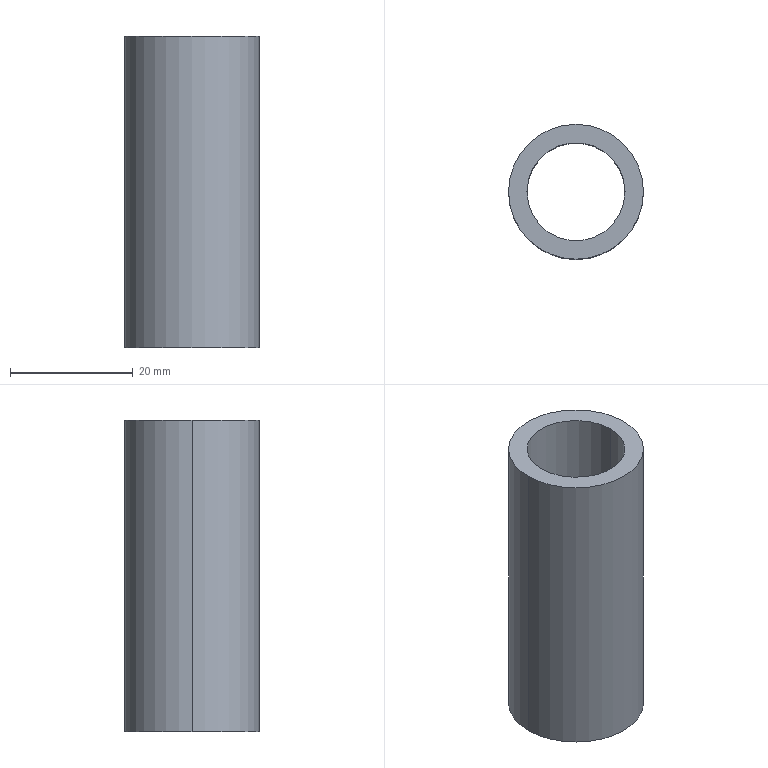Part | SolidWorks | features Extrusion 1 | 1 solid | 6 faces | box 22 x 22 x 50.8 mm | volume 9097 mm3 | cylinder 4 | plane 2 | commonest cylinder face diameters 16 x2 22 x2
STEP:
#1=CARTESIAN_POINT('',(-8.,0.,50.8));
#2=VERTEX_POINT('',#1);
#3=CARTESIAN_POINT('',(8.,0.,50.8));
#4=VERTEX_POINT('',#3);
#5=CARTESIAN_POINT('',(0.,0.,50.8));
#6=DIRECTION('',(0.,0.,1.));
#7=DIRECTION('',(1.,0.,0.));
#8=AXIS2_PLACEMENT_3D('',#5,#6,#7);
#9=CIRCLE('',#8,8.);
#10=EDGE_CURVE('',#2,#4,#9,.T.);
#11=ORIENTED_EDGE('',*,*,#10,.T.);
#12=CARTESIAN_POINT('',(8.,0.,0.));
#13=VERTEX_POINT('',#12);
#14=CARTESIAN_POINT('',(8.,0.,50.8));
#15=DIRECTION('',(0.,0.,-1.));
#16=VECTOR('',#15,1000.);
#17=LINE('',#14,#16);
#18=EDGE_CURVE('',#4,#13,#17,.T.);
#19=ORIENTED_EDGE('',*,*,#18,.T.);
#20=CARTESIAN_POINT('',(-8.,0.,0.));
#21=VERTEX_POINT('',#20);
#22=CARTESIAN_POINT('',(0.,0.,0.));
#23=DIRECTION('',(0.,0.,1.));
#24=DIRECTION('',(1.,0.,0.));
#25=AXIS2_PLACEMENT_3D('',#22,#23,#24);
#26=CIRCLE('',#25,8.);
#27=EDGE_CURVE('',#21,#13,#26,.T.);
#28=ORIENTED_EDGE('',*,*,#27,.F.);
#29=CARTESIAN_POINT('',(-8.,0.,50.8));
#30=DIRECTION('',(0.,0.,-1.));
#31=VECTOR('',#30,1000.);
#32=LINE('',#29,#31);
#33=EDGE_CURVE('',#2,#21,#32,.T.);
#34=ORIENTED_EDGE('',*,*,#33,.F.);
#35=EDGE_LOOP('',(#11,#19,#28,#34));
#36=FACE_OUTER_BOUND('',#35,.T.);
#37=CARTESIAN_POINT('',(0.,0.,50.8));
#38=DIRECTION('',(0.,0.,-1.));
#39=DIRECTION('',(-1.,0.,0.));
#40=AXIS2_PLACEMENT_3D('',#37,#38,#39);
#41=CYLINDRICAL_SURFACE('',#40,8.);
#42=ADVANCED_FACE('',(#36),#41,.F.);
#43=CARTESIAN_POINT('',(11.,0.,50.8));
#44=VERTEX_POINT('',#43);
#45=CARTESIAN_POINT('',(-11.,0.,50.8));
#46=VERTEX_POINT('',#45);
#47=CARTESIAN_POINT('',(0.,0.,50.8));
#48=DIRECTION('',(0.,0.,1.));
#49=DIRECTION('',(1.,0.,0.));
#50=AXIS2_PLACEMENT_3D('',#47,#48,#49);
#51=CIRCLE('',#50,11.);
#52=EDGE_CURVE('',#44,#46,#51,.T.);
#53=ORIENTED_EDGE('',*,*,#52,.F.);
#54=CARTESIAN_POINT('',(11.,0.,0.));
#55=VERTEX_POINT('',#54);
#56=CARTESIAN_POINT('',(11.,0.,50.8));
#57=DIRECTION('',(0.,0.,-1.));
#58=VECTOR('',#57,1000.);
#59=LINE('',#56,#58);
#60=EDGE_CURVE('',#44,#55,#59,.T.);
#61=ORIENTED_EDGE('',*,*,#60,.T.);
#62=CARTESIAN_POINT('',(-11.,0.,0.));
#63=VERTEX_POINT('',#62);
#64=CARTESIAN_POINT('',(0.,0.,0.));
#65=DIRECTION('',(0.,0.,1.));
#66=DIRECTION('',(1.,0.,0.));
#67=AXIS2_PLACEMENT_3D('',#64,#65,#66);
#68=CIRCLE('',#67,11.);
#69=EDGE_CURVE('',#55,#63,#68,.T.);
#70=ORIENTED_EDGE('',*,*,#69,.T.);
#71=CARTESIAN_POINT('',(-11.,0.,50.8));
#72=DIRECTION('',(0.,0.,-1.));
#73=VECTOR('',#72,1000.);
#74=LINE('',#71,#73);
#75=EDGE_CURVE('',#46,#63,#74,.T.);
#76=ORIENTED_EDGE('',*,*,#75,.F.);
#77=EDGE_LOOP('',(#53,#61,#70,#76));
#78=FACE_OUTER_BOUND('',#77,.T.);
#79=CARTESIAN_POINT('',(0.,0.,50.8));
#80=DIRECTION('',(0.,0.,-1.));
#81=DIRECTION('',(-1.,0.,0.));
#82=AXIS2_PLACEMENT_3D('',#79,#80,#81);
#83=CYLINDRICAL_SURFACE('',#82,11.);
#84=ADVANCED_FACE('',(#78),#83,.T.);
#85=CARTESIAN_POINT('',(0.,0.,50.8));
#86=DIRECTION('',(0.,0.,1.));
#87=DIRECTION('',(1.,0.,0.));
#88=AXIS2_PLACEMENT_3D('',#85,#86,#87);
#89=CIRCLE('',#88,11.);
#90=EDGE_CURVE('',#46,#44,#89,.T.);
#91=ORIENTED_EDGE('',*,*,#90,.T.);
#92=ORIENTED_EDGE('',*,*,#52,.T.);
#93=EDGE_LOOP('',(#91,#92));
#94=FACE_OUTER_BOUND('',#93,.T.);
#95=ORIENTED_EDGE('',*,*,#10,.F.);
#96=CARTESIAN_POINT('',(0.,0.,50.8));
#97=DIRECTION('',(0.,0.,1.));
#98=DIRECTION('',(1.,0.,0.));
#99=AXIS2_PLACEMENT_3D('',#96,#97,#98);
#100=CIRCLE('',#99,8.);
#101=EDGE_CURVE('',#4,#2,#100,.T.);
#102=ORIENTED_EDGE('',*,*,#101,.F.);
#103=EDGE_LOOP('',(#95,#102));
#104=FACE_BOUND('',#103,.T.);
#105=CARTESIAN_POINT('',(0.,0.,50.8));
#106=DIRECTION('',(0.,0.,1.));
#107=DIRECTION('',(1.,0.,0.));
#108=AXIS2_PLACEMENT_3D('',#105,#106,#107);
#109=PLANE('',#108);
#110=ADVANCED_FACE('',(#94,#104),#109,.T.);
#111=CARTESIAN_POINT('',(0.,0.,0.));
#112=DIRECTION('',(0.,0.,1.));
#113=DIRECTION('',(1.,0.,0.));
#114=AXIS2_PLACEMENT_3D('',#111,#112,#113);
#115=CIRCLE('',#114,11.);
#116=EDGE_CURVE('',#63,#55,#115,.T.);
#117=ORIENTED_EDGE('',*,*,#116,.F.);
#118=ORIENTED_EDGE('',*,*,#69,.F.);
#119=EDGE_LOOP('',(#117,#118));
#120=FACE_OUTER_BOUND('',#119,.T.);
#121=ORIENTED_EDGE('',*,*,#27,.T.);
#122=CARTESIAN_POINT('',(0.,0.,0.));
#123=DIRECTION('',(0.,0.,1.));
#124=DIRECTION('',(1.,0.,0.));
#125=AXIS2_PLACEMENT_3D('',#122,#123,#124);
#126=CIRCLE('',#125,8.);
#127=EDGE_CURVE('',#13,#21,#126,.T.);
#128=ORIENTED_EDGE('',*,*,#127,.T.);
#129=EDGE_LOOP('',(#121,#128));
#130=FACE_BOUND('',#129,.T.);
#131=CARTESIAN_POINT('',(0.,0.,0.));
#132=DIRECTION('',(0.,0.,1.));
#133=DIRECTION('',(1.,0.,0.));
#134=AXIS2_PLACEMENT_3D('',#131,#132,#133);
#135=PLANE('',#134);
#136=ADVANCED_FACE('',(#120,#130),#135,.F.);
#137=ORIENTED_EDGE('',*,*,#60,.F.);
#138=ORIENTED_EDGE('',*,*,#90,.F.);
#139=ORIENTED_EDGE('',*,*,#75,.T.);
#140=ORIENTED_EDGE('',*,*,#116,.T.);
#141=EDGE_LOOP('',(#137,#138,#139,#140));
#142=FACE_OUTER_BOUND('',#141,.T.);
#143=CARTESIAN_POINT('',(0.,0.,50.8));
#144=DIRECTION('',(0.,0.,-1.));
#145=DIRECTION('',(-1.,0.,0.));
#146=AXIS2_PLACEMENT_3D('',#143,#144,#145);
#147=CYLINDRICAL_SURFACE('',#146,11.);
#148=ADVANCED_FACE('',(#142),#147,.T.);
#149=ORIENTED_EDGE('',*,*,#18,.F.);
#150=ORIENTED_EDGE('',*,*,#101,.T.);
#151=ORIENTED_EDGE('',*,*,#33,.T.);
#152=ORIENTED_EDGE('',*,*,#127,.F.);
#153=EDGE_LOOP('',(#149,#150,#151,#152));
#154=FACE_OUTER_BOUND('',#153,.T.);
#155=CARTESIAN_POINT('',(0.,0.,50.8));
#156=DIRECTION('',(0.,0.,-1.));
#157=DIRECTION('',(-1.,0.,0.));
#158=AXIS2_PLACEMENT_3D('',#155,#156,#157);
#159=CYLINDRICAL_SURFACE('',#158,8.);
#160=ADVANCED_FACE('',(#154),#159,.F.);
#161=CLOSED_SHELL('',(#42,#84,#110,#136,#148,#160));
#162=MANIFOLD_SOLID_BREP('',#161);
#163=CARTESIAN_POINT('',(0.,0.,0.));
#164=DIRECTION('',(0.,0.,1.));
#165=DIRECTION('',(1.,0.,0.));
#166=AXIS2_PLACEMENT_3D('',#163,#164,#165);
#167=(LENGTH_UNIT()NAMED_UNIT(*)SI_UNIT(.MILLI.,.METRE.));
#168=UNCERTAINTY_MEASURE_WITH_UNIT(LENGTH_MEASURE(0.00001),#167,'','');
#169=(NAMED_UNIT(*)PLANE_ANGLE_UNIT()SI_UNIT($,.RADIAN.));
#170=(NAMED_UNIT(*)SI_UNIT($,.STERADIAN.)SOLID_ANGLE_UNIT());
#171=(GEOMETRIC_REPRESENTATION_CONTEXT(3)GLOBAL_UNCERTAINTY_ASSIGNED_CONTEXT((#168))GLOBAL_UNIT_ASSIGNED_CONTEXT((#167,#169,#170))REPRESENTATION_CONTEXT('',''));
#172=ADVANCED_BREP_SHAPE_REPRESENTATION('',(#162,#166),#171);